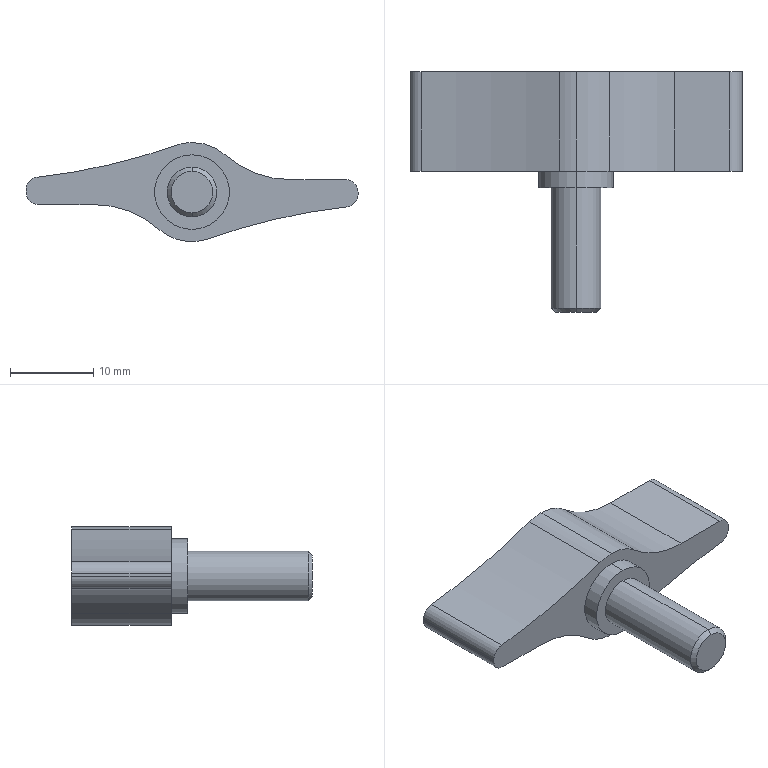Part | SolidWorks | features ICE 10, Fillet 6, BaseBody 1, Chamfer 1, HoleWzd 1, MoveCopyBody 1, Stock 1 | 2 solids | 59 faces | box 40 x 29 x 11.94 mm | volume 3436 mm3 | plane 24 | cylinder 23 | cone 8 | torus 4 | commonest cylinder face diameters 3 x4 12 x3 4 x2 4.3 x2 6 x2 7 x2